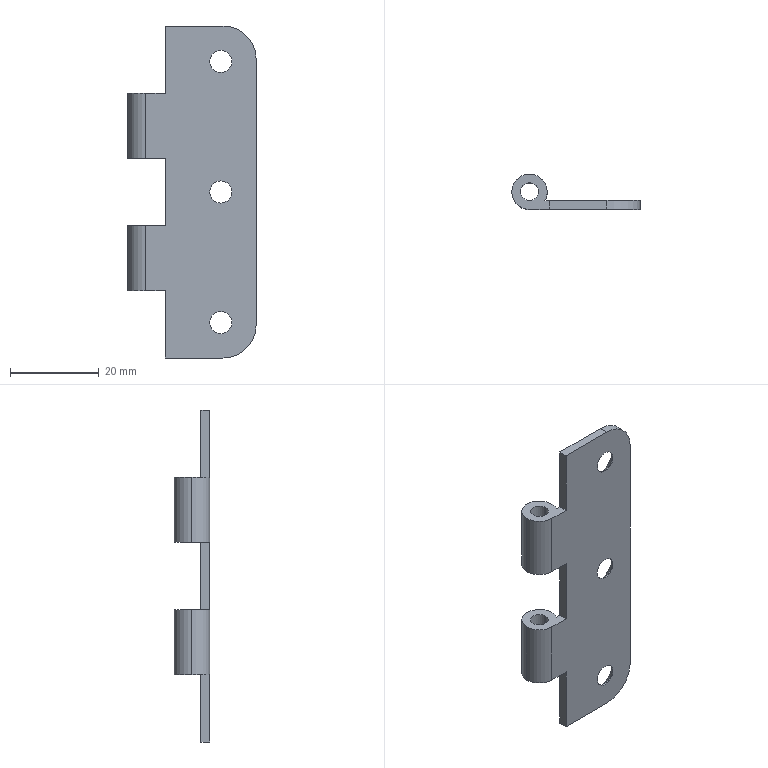Part | STEP file | 1 solid | 36 faces | box 29 x 8 x 75 mm | volume 4043 mm3 | cylinder 18 | plane 12 | cone 6 | commonest cylinder face diameters 5 x6 8 x6 4 x4 15 x2